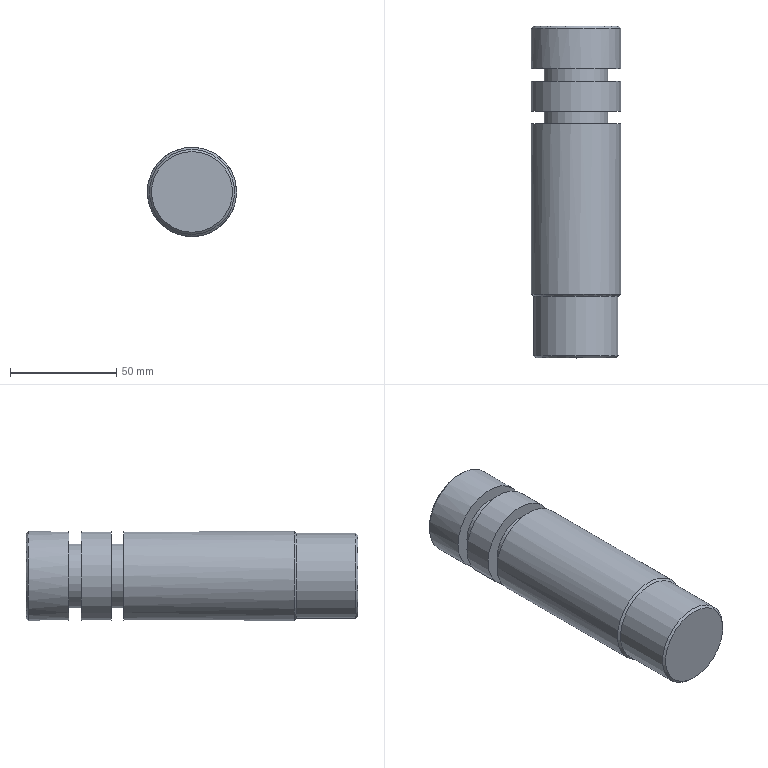Part | NX | features solid 2 | 1 solid | 15 faces | box 42 x 156 x 42 mm | volume 204059 mm3 | plane 6 | cylinder 6 | cone 3 | commonest cylinder face diameters 42 x3 30 x2 40 x1
STEP:
#1=CARTESIAN_POINT('',(1131.,445.,180.));
#2=VERTEX_POINT('',#1);
#3=CARTESIAN_POINT('',(1110.,445.,180.));
#4=DIRECTION('',(0.,-1.,0.));
#5=DIRECTION('',(1.,0.,0.));
#6=AXIS2_PLACEMENT_3D('',#3,#4,#5);
#7=CIRCLE('',#6,21.);
#8=EDGE_CURVE('',#2,#2,#7,.T.);
#9=ORIENTED_EDGE('',*,*,#8,.F.);
#10=EDGE_LOOP('',(#9));
#11=FACE_BOUND('',#10,.T.);
#12=CARTESIAN_POINT('',(1125.,445.,180.));
#13=VERTEX_POINT('',#12);
#14=CARTESIAN_POINT('',(1110.,445.,180.));
#15=DIRECTION('',(0.,-1.,0.));
#16=DIRECTION('',(1.,0.,0.));
#17=AXIS2_PLACEMENT_3D('',#14,#15,#16);
#18=CIRCLE('',#17,15.);
#19=EDGE_CURVE('',#13,#13,#18,.T.);
#20=ORIENTED_EDGE('',*,*,#19,.T.);
#21=EDGE_LOOP('',(#20));
#22=FACE_BOUND('',#21,.T.);
#23=CARTESIAN_POINT('',(1110.,445.,180.));
#24=DIRECTION('',(0.,1.,0.));
#25=DIRECTION('',(0.,0.,-1.));
#26=AXIS2_PLACEMENT_3D('',#23,#24,#25);
#27=PLANE('',#26);
#28=ADVANCED_FACE('',(#11,#22),#27,.T.);
#29=CARTESIAN_POINT('',(1131.,425.,180.));
#30=VERTEX_POINT('',#29);
#31=CARTESIAN_POINT('',(1110.,425.,180.));
#32=DIRECTION('',(0.,-1.,0.));
#33=DIRECTION('',(1.,0.,0.));
#34=AXIS2_PLACEMENT_3D('',#31,#32,#33);
#35=CIRCLE('',#34,21.);
#36=EDGE_CURVE('',#30,#30,#35,.T.);
#37=ORIENTED_EDGE('',*,*,#36,.F.);
#38=EDGE_LOOP('',(#37));
#39=FACE_BOUND('',#38,.T.);
#40=CARTESIAN_POINT('',(1125.,425.,180.));
#41=VERTEX_POINT('',#40);
#42=CARTESIAN_POINT('',(1110.,425.,180.));
#43=DIRECTION('',(0.,-1.,0.));
#44=DIRECTION('',(1.,0.,0.));
#45=AXIS2_PLACEMENT_3D('',#42,#43,#44);
#46=CIRCLE('',#45,15.);
#47=EDGE_CURVE('',#41,#41,#46,.T.);
#48=ORIENTED_EDGE('',*,*,#47,.T.);
#49=EDGE_LOOP('',(#48));
#50=FACE_BOUND('',#49,.T.);
#51=CARTESIAN_POINT('',(1110.,425.,180.));
#52=DIRECTION('',(0.,1.,0.));
#53=DIRECTION('',(0.,0.,-1.));
#54=AXIS2_PLACEMENT_3D('',#51,#52,#53);
#55=PLANE('',#54);
#56=ADVANCED_FACE('',(#39,#50),#55,.T.);
#57=CARTESIAN_POINT('',(1131.,345.,180.));
#58=VERTEX_POINT('',#57);
#59=CARTESIAN_POINT('',(1110.,345.,180.));
#60=DIRECTION('',(0.,-1.,0.));
#61=DIRECTION('',(1.,0.,0.));
#62=AXIS2_PLACEMENT_3D('',#59,#60,#61);
#63=CIRCLE('',#62,21.);
#64=EDGE_CURVE('',#58,#58,#63,.T.);
#65=ORIENTED_EDGE('',*,*,#64,.F.);
#66=EDGE_LOOP('',(#65));
#67=FACE_BOUND('',#66,.T.);
#68=ORIENTED_EDGE('',*,*,#36,.T.);
#69=EDGE_LOOP('',(#68));
#70=FACE_BOUND('',#69,.T.);
#71=CARTESIAN_POINT('',(1110.,405.,180.));
#72=DIRECTION('',(0.,-1.,0.));
#73=DIRECTION('',(0.,0.,1.));
#74=AXIS2_PLACEMENT_3D('',#71,#72,#73);
#75=CYLINDRICAL_SURFACE('',#74,21.);
#76=ADVANCED_FACE('',(#67,#70),#75,.T.);
#77=CARTESIAN_POINT('',(1125.,431.,180.));
#78=VERTEX_POINT('',#77);
#79=CARTESIAN_POINT('',(1110.,431.,180.));
#80=DIRECTION('',(0.,-1.,0.));
#81=DIRECTION('',(1.,0.,0.));
#82=AXIS2_PLACEMENT_3D('',#79,#80,#81);
#83=CIRCLE('',#82,15.);
#84=EDGE_CURVE('',#78,#78,#83,.T.);
#85=ORIENTED_EDGE('',*,*,#84,.T.);
#86=EDGE_LOOP('',(#85));
#87=FACE_BOUND('',#86,.T.);
#88=ORIENTED_EDGE('',*,*,#47,.F.);
#89=EDGE_LOOP('',(#88));
#90=FACE_BOUND('',#89,.T.);
#91=CARTESIAN_POINT('',(1110.,431.,180.));
#92=DIRECTION('',(0.,-1.,0.));
#93=DIRECTION('',(0.,0.,1.));
#94=AXIS2_PLACEMENT_3D('',#91,#92,#93);
#95=CYLINDRICAL_SURFACE('',#94,15.);
#96=ADVANCED_FACE('',(#87,#90),#95,.T.);
#97=CARTESIAN_POINT('',(1131.,431.,180.));
#98=VERTEX_POINT('',#97);
#99=CARTESIAN_POINT('',(1110.,431.,180.));
#100=DIRECTION('',(0.,-1.,0.));
#101=DIRECTION('',(1.,0.,0.));
#102=AXIS2_PLACEMENT_3D('',#99,#100,#101);
#103=CIRCLE('',#102,21.);
#104=EDGE_CURVE('',#98,#98,#103,.T.);
#105=ORIENTED_EDGE('',*,*,#104,.T.);
#106=EDGE_LOOP('',(#105));
#107=FACE_BOUND('',#106,.T.);
#108=ORIENTED_EDGE('',*,*,#84,.F.);
#109=EDGE_LOOP('',(#108));
#110=FACE_BOUND('',#109,.T.);
#111=CARTESIAN_POINT('',(1110.,431.,180.));
#112=DIRECTION('',(0.,1.,0.));
#113=DIRECTION('',(0.,0.,-1.));
#114=AXIS2_PLACEMENT_3D('',#111,#112,#113);
#115=PLANE('',#114);
#116=ADVANCED_FACE('',(#107,#110),#115,.F.);
#117=ORIENTED_EDGE('',*,*,#8,.T.);
#118=EDGE_LOOP('',(#117));
#119=FACE_BOUND('',#118,.T.);
#120=ORIENTED_EDGE('',*,*,#104,.F.);
#121=EDGE_LOOP('',(#120));
#122=FACE_BOUND('',#121,.T.);
#123=CARTESIAN_POINT('',(1110.,445.,180.));
#124=DIRECTION('',(0.,-1.,0.));
#125=DIRECTION('',(0.,0.,1.));
#126=AXIS2_PLACEMENT_3D('',#123,#124,#125);
#127=CYLINDRICAL_SURFACE('',#126,21.);
#128=ADVANCED_FACE('',(#119,#122),#127,.T.);
#129=CARTESIAN_POINT('',(1125.,451.,180.));
#130=VERTEX_POINT('',#129);
#131=CARTESIAN_POINT('',(1110.,451.,180.));
#132=DIRECTION('',(0.,-1.,0.));
#133=DIRECTION('',(1.,0.,0.));
#134=AXIS2_PLACEMENT_3D('',#131,#132,#133);
#135=CIRCLE('',#134,15.);
#136=EDGE_CURVE('',#130,#130,#135,.T.);
#137=ORIENTED_EDGE('',*,*,#136,.T.);
#138=EDGE_LOOP('',(#137));
#139=FACE_BOUND('',#138,.T.);
#140=ORIENTED_EDGE('',*,*,#19,.F.);
#141=EDGE_LOOP('',(#140));
#142=FACE_BOUND('',#141,.T.);
#143=CARTESIAN_POINT('',(1110.,451.,180.));
#144=DIRECTION('',(0.,-1.,0.));
#145=DIRECTION('',(0.,0.,1.));
#146=AXIS2_PLACEMENT_3D('',#143,#144,#145);
#147=CYLINDRICAL_SURFACE('',#146,15.);
#148=ADVANCED_FACE('',(#139,#142),#147,.T.);
#149=CARTESIAN_POINT('',(1131.,451.,180.));
#150=VERTEX_POINT('',#149);
#151=CARTESIAN_POINT('',(1110.,451.,180.));
#152=DIRECTION('',(0.,-1.,0.));
#153=DIRECTION('',(1.,0.,0.));
#154=AXIS2_PLACEMENT_3D('',#151,#152,#153);
#155=CIRCLE('',#154,21.);
#156=EDGE_CURVE('',#150,#150,#155,.T.);
#157=ORIENTED_EDGE('',*,*,#156,.T.);
#158=EDGE_LOOP('',(#157));
#159=FACE_BOUND('',#158,.T.);
#160=ORIENTED_EDGE('',*,*,#136,.F.);
#161=EDGE_LOOP('',(#160));
#162=FACE_BOUND('',#161,.T.);
#163=CARTESIAN_POINT('',(1110.,451.,180.));
#164=DIRECTION('',(0.,1.,0.));
#165=DIRECTION('',(0.,0.,-1.));
#166=AXIS2_PLACEMENT_3D('',#163,#164,#165);
#167=PLANE('',#166);
#168=ADVANCED_FACE('',(#159,#162),#167,.F.);
#169=CARTESIAN_POINT('',(1110.,470.,159.));
#170=VERTEX_POINT('',#169);
#171=CARTESIAN_POINT('',(1110.,470.,180.));
#172=DIRECTION('',(0.,-1.,0.));
#173=DIRECTION('',(0.,0.,-1.));
#174=AXIS2_PLACEMENT_3D('',#171,#172,#173);
#175=CIRCLE('',#174,21.);
#176=EDGE_CURVE('',#170,#170,#175,.F.);
#177=ORIENTED_EDGE('',*,*,#176,.F.);
#178=EDGE_LOOP('',(#177));
#179=FACE_BOUND('',#178,.T.);
#180=ORIENTED_EDGE('',*,*,#156,.F.);
#181=EDGE_LOOP('',(#180));
#182=FACE_BOUND('',#181,.T.);
#183=CARTESIAN_POINT('',(1110.,471.,180.));
#184=DIRECTION('',(0.,-1.,0.));
#185=DIRECTION('',(0.,0.,1.));
#186=AXIS2_PLACEMENT_3D('',#183,#184,#185);
#187=CYLINDRICAL_SURFACE('',#186,21.);
#188=ADVANCED_FACE('',(#179,#182),#187,.T.);
#189=CARTESIAN_POINT('',(1110.,471.,160.));
#190=VERTEX_POINT('',#189);
#191=CARTESIAN_POINT('',(1110.,471.,180.));
#192=DIRECTION('',(0.,-1.,0.));
#193=DIRECTION('',(0.,0.,-1.));
#194=AXIS2_PLACEMENT_3D('',#191,#192,#193);
#195=CIRCLE('',#194,20.);
#196=EDGE_CURVE('',#190,#190,#195,.T.);
#197=ORIENTED_EDGE('',*,*,#196,.F.);
#198=EDGE_LOOP('',(#197));
#199=FACE_BOUND('',#198,.T.);
#200=CARTESIAN_POINT('',(1110.,471.,180.));
#201=DIRECTION('',(0.,1.,0.));
#202=DIRECTION('',(0.,0.,-1.));
#203=AXIS2_PLACEMENT_3D('',#200,#201,#202);
#204=PLANE('',#203);
#205=ADVANCED_FACE('',(#199),#204,.T.);
#206=CARTESIAN_POINT('',(1110.,344.,160.));
#207=VERTEX_POINT('',#206);
#208=CARTESIAN_POINT('',(1110.,344.,180.));
#209=DIRECTION('',(0.,-1.,0.));
#210=DIRECTION('',(0.,0.,-1.));
#211=AXIS2_PLACEMENT_3D('',#208,#209,#210);
#212=CIRCLE('',#211,20.);
#213=EDGE_CURVE('',#207,#207,#212,.F.);
#214=ORIENTED_EDGE('',*,*,#213,.F.);
#215=EDGE_LOOP('',(#214));
#216=FACE_BOUND('',#215,.T.);
#217=CARTESIAN_POINT('',(1110.,316.,160.));
#218=VERTEX_POINT('',#217);
#219=CARTESIAN_POINT('',(1110.,316.,180.));
#220=DIRECTION('',(0.,-1.,0.));
#221=DIRECTION('',(0.,0.,-1.));
#222=AXIS2_PLACEMENT_3D('',#219,#220,#221);
#223=CIRCLE('',#222,20.);
#224=EDGE_CURVE('',#218,#218,#223,.T.);
#225=ORIENTED_EDGE('',*,*,#224,.F.);
#226=EDGE_LOOP('',(#225));
#227=FACE_BOUND('',#226,.T.);
#228=CARTESIAN_POINT('',(1110.,275.,180.));
#229=DIRECTION('',(0.,1.,0.));
#230=DIRECTION('',(0.,0.,-1.));
#231=AXIS2_PLACEMENT_3D('',#228,#229,#230);
#232=CYLINDRICAL_SURFACE('',#231,20.);
#233=ADVANCED_FACE('',(#216,#227),#232,.T.);
#234=CARTESIAN_POINT('',(1110.,315.,161.));
#235=VERTEX_POINT('',#234);
#236=CARTESIAN_POINT('',(1110.,315.,180.));
#237=DIRECTION('',(0.,-1.,0.));
#238=DIRECTION('',(0.,0.,-1.));
#239=AXIS2_PLACEMENT_3D('',#236,#237,#238);
#240=CIRCLE('',#239,19.);
#241=EDGE_CURVE('',#235,#235,#240,.F.);
#242=ORIENTED_EDGE('',*,*,#241,.F.);
#243=EDGE_LOOP('',(#242));
#244=FACE_BOUND('',#243,.T.);
#245=CARTESIAN_POINT('',(1110.,315.,180.));
#246=DIRECTION('',(0.,1.,0.));
#247=DIRECTION('',(0.,0.,-1.));
#248=AXIS2_PLACEMENT_3D('',#245,#246,#247);
#249=PLANE('',#248);
#250=ADVANCED_FACE('',(#244),#249,.F.);
#251=ORIENTED_EDGE('',*,*,#241,.T.);
#252=EDGE_LOOP('',(#251));
#253=FACE_BOUND('',#252,.T.);
#254=ORIENTED_EDGE('',*,*,#224,.T.);
#255=EDGE_LOOP('',(#254));
#256=FACE_BOUND('',#255,.T.);
#257=CARTESIAN_POINT('',(1110.,316.,180.));
#258=DIRECTION('',(0.,1.,0.));
#259=DIRECTION('',(0.,0.,-1.));
#260=AXIS2_PLACEMENT_3D('',#257,#258,#259);
#261=CONICAL_SURFACE('',#260,20.,0.7854);
#262=ADVANCED_FACE('',(#253,#256),#261,.T.);
#263=ORIENTED_EDGE('',*,*,#213,.T.);
#264=EDGE_LOOP('',(#263));
#265=FACE_BOUND('',#264,.T.);
#266=ORIENTED_EDGE('',*,*,#64,.T.);
#267=EDGE_LOOP('',(#266));
#268=FACE_BOUND('',#267,.T.);
#269=CARTESIAN_POINT('',(1110.,345.,180.));
#270=DIRECTION('',(0.,1.,0.));
#271=DIRECTION('',(0.,0.,-1.));
#272=AXIS2_PLACEMENT_3D('',#269,#270,#271);
#273=CONICAL_SURFACE('',#272,21.,0.7854);
#274=ADVANCED_FACE('',(#265,#268),#273,.T.);
#275=ORIENTED_EDGE('',*,*,#176,.T.);
#276=EDGE_LOOP('',(#275));
#277=FACE_BOUND('',#276,.T.);
#278=ORIENTED_EDGE('',*,*,#196,.T.);
#279=EDGE_LOOP('',(#278));
#280=FACE_BOUND('',#279,.T.);
#281=CARTESIAN_POINT('',(1110.,471.,180.));
#282=DIRECTION('',(0.,-1.,0.));
#283=DIRECTION('',(0.,0.,1.));
#284=AXIS2_PLACEMENT_3D('',#281,#282,#283);
#285=CONICAL_SURFACE('',#284,20.,0.7854);
#286=ADVANCED_FACE('',(#277,#280),#285,.T.);
#287=CLOSED_SHELL('',(#28,#56,#76,#96,#116,#128,#148,#168,#188,#205,#233,#250,#262,#274,#286));
#288=MANIFOLD_SOLID_BREP('',#287);
#289=(LENGTH_UNIT()NAMED_UNIT(*)SI_UNIT(.MILLI.,.METRE.));
#290=UNCERTAINTY_MEASURE_WITH_UNIT(LENGTH_MEASURE(0.00001),#289,'','');
#291=(NAMED_UNIT(*)PLANE_ANGLE_UNIT()SI_UNIT($,.RADIAN.));
#292=(NAMED_UNIT(*)SI_UNIT($,.STERADIAN.)SOLID_ANGLE_UNIT());
#293=(GEOMETRIC_REPRESENTATION_CONTEXT(3)GLOBAL_UNCERTAINTY_ASSIGNED_CONTEXT((#290))GLOBAL_UNIT_ASSIGNED_CONTEXT((#289,#291,#292))REPRESENTATION_CONTEXT('',''));
#294=ADVANCED_BREP_SHAPE_REPRESENTATION('',(#288),#293);